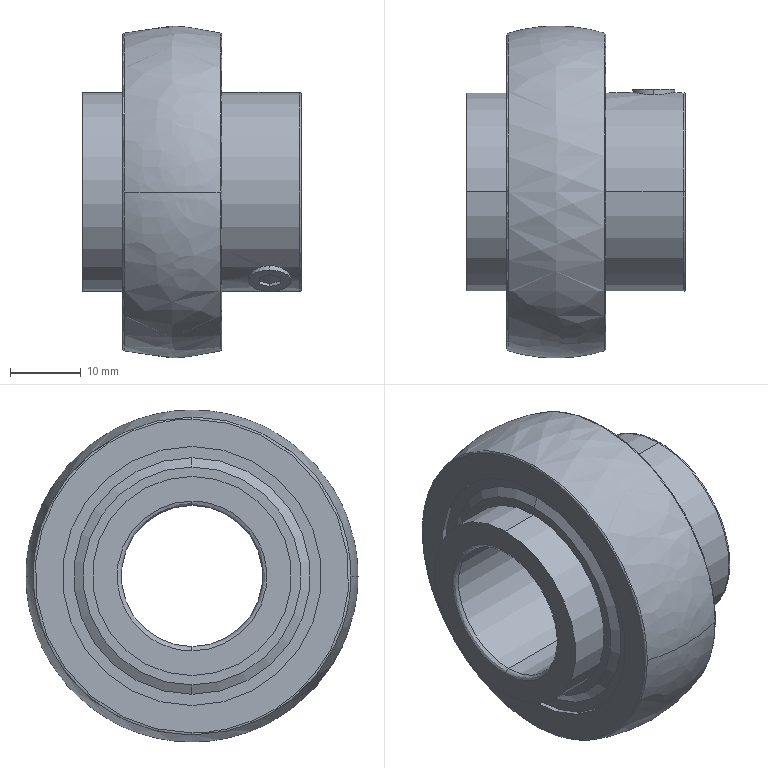Part | STEP file | Microwave Drying Flat Conveyor-YAR 204-2FW_VA228_Default | 1 solid | 54 faces | box 31 x 47 x 47 mm | volume 24116 mm3 | plane 22 | cylinder 16 | spline 12 | cone 4 | commonest cylinder face diameters 28.2 x6 6 x4 36.675 x4 20 x2